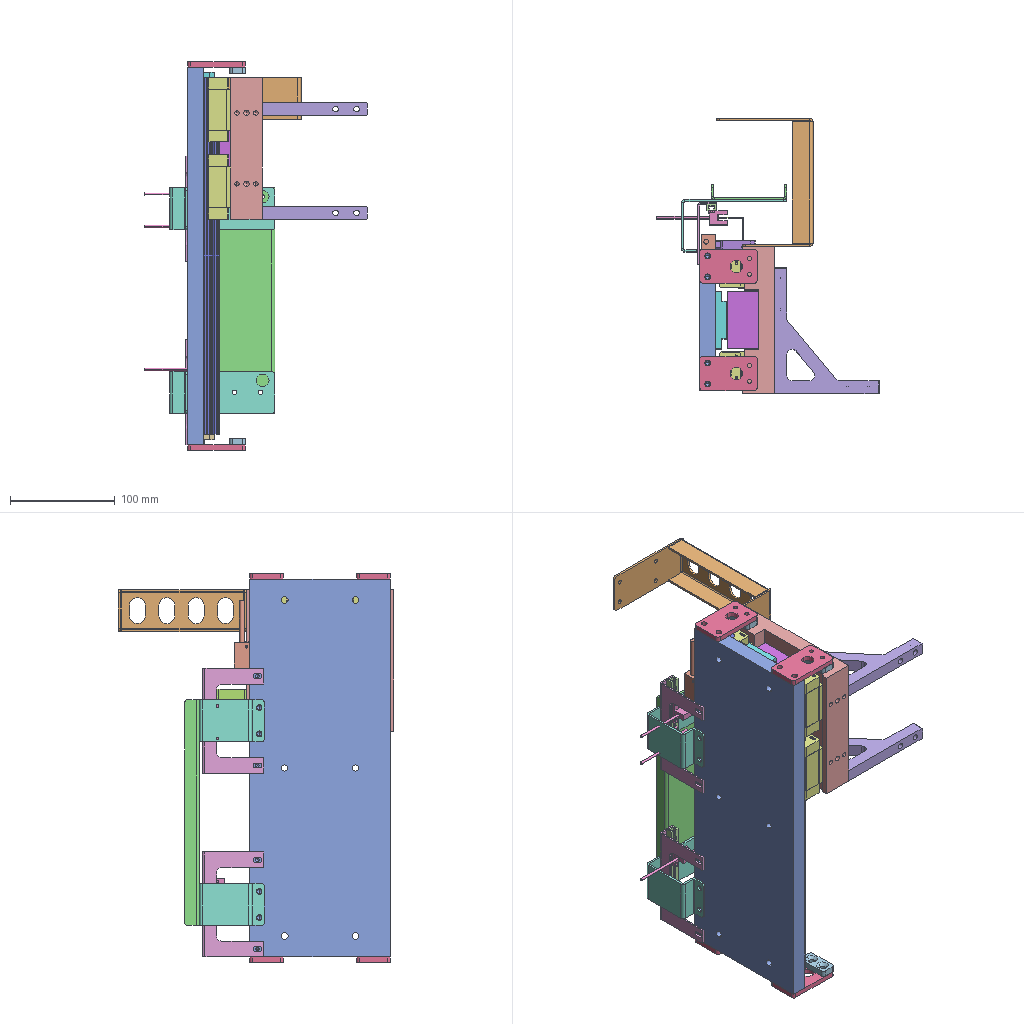Assembly | SolidWorks | 21 different items | 37 placed | box 212 x 262 x 370 mm
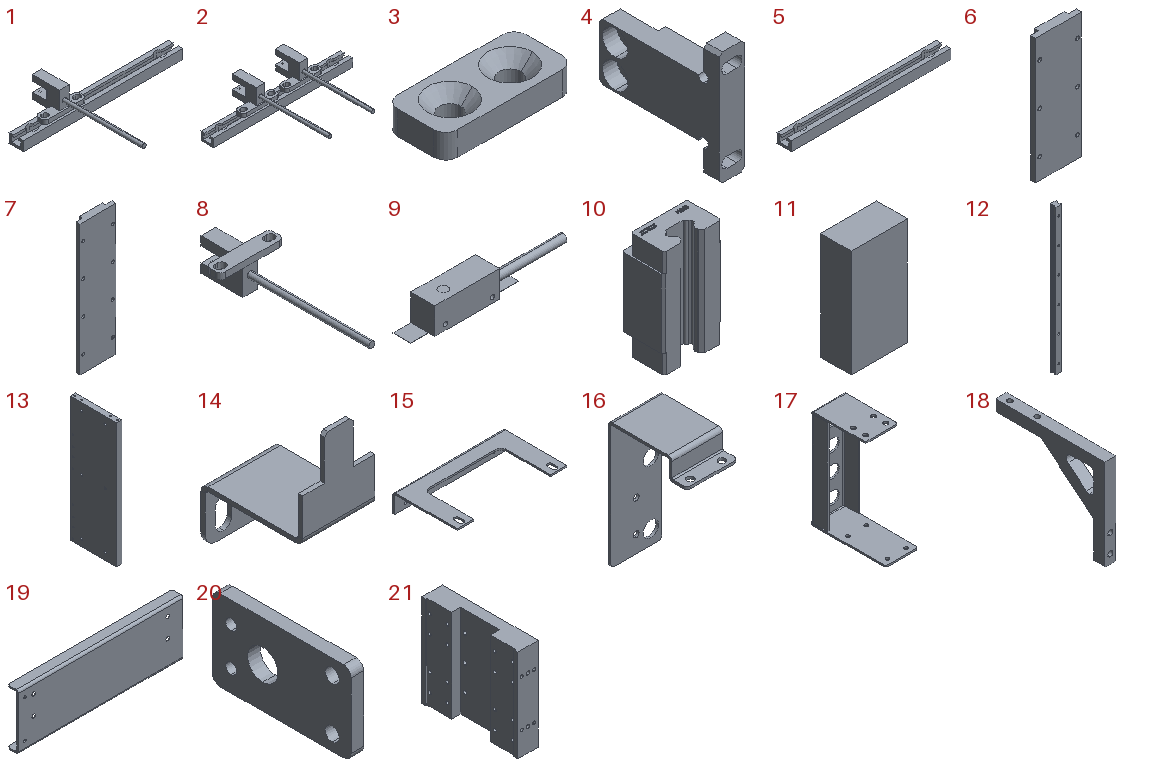Parts list (item | name | quantity | parent item | size | volume | features):
1 | (subassembly) | x1 | - | 100 x 67.2 x 19.7 mm | 4708 mm3 | -
2 | (subassembly) | x1 | - | 100 x 67.2 x 19.7 mm | 6293 mm3 | -
3 | - | x4 | - | 32 x 15 x 6 mm | 2360 mm3 | features Extrusion 1, Fillet 1, HoleWzd 1
4 | - | x1 | - | 8 x 38 x 36 mm | 4843 mm3 | features HoleWzd 2, ICE 2, Chamfer 1, Extrusion 1
5 | - | x2 | in 1, 2 | 100 x 9 x 6 mm | 3122 mm3 | features BaseBody 1
6 | - | x1 | - | 55 x 10.7 x 150 mm | 73163 mm3 | features BaseBody 1
7 | - | x1 | - | 55 x 10.7 x 200 mm | 97550 mm3 | features BaseBody 1
8 | - | x3 | in 1, 2 | 26 x 67.2 x 13.7 mm | 1586 mm3 | features BaseBody 1
9 | - | x1 | - | 86 x 13.4 x 14.9 mm | 7701 mm3 | features BaseBody 2
10 | - | x4 | - | 34 x 23.7 x 61.7 mm | 37046 mm3 | features BaseBody 1
11 | - | x1 | - | 55 x 30 x 120 mm | 172847 mm3 | features BaseBody 1
12 | - | x2 | - | 15 x 15 x 340 mm | 62525 mm3 | features Extrusion 1, HoleWzd 1, ICE 1, LPattern 1
13 | - | x1 | - | 15 x 134 x 360 mm | 714258 mm3 | features HoleWzd 7, LPattern 2, Extrusion 1, MirrorPattern 1
14 | - | x1 | - | 20 x 28.2 x 38 mm | 1272 mm3 | features Chamfer 1, Cut 1, Fillet 1, FlatPattern 1, HoleWzd 1, SMBaseFlange 1, SheetMetal 1
15 | - | x2 | - | 100 x 58.5 x 17.5 mm | 6237 mm3 | features HoleWzd 2, Cut 1, FlatPattern 1, SMBaseFlange 1, SheetMetal 1
16 | - | x2 | - | 40 x 62 x 100 mm | 13167 mm3 | features HoleWzd 3, Fillet 1, FlatPattern 1, SMBaseFlange 1, SheetMetal 1
17 | - | x1 | - | 40 x 92 x 122 mm | 27046 mm3 | features HoleWzd 2, EdgeFlange 1, Fillet 1, FlatPattern 1, ICE 1, LPattern 1, SMBaseFlange 1, SheetMetal 1
18 | - | x2 | - | 12 x 120 x 100 mm | 37463 mm3 | features HoleWzd 2, Chamfer 1, Extrusion 1, Fillet 1, ICE 1
19 | - | x1 | - | 215 x 14 x 72 mm | 40210 mm3 | features HoleWzd 2, Fillet 1, FlatPattern 1, SMBaseFlange 1, SheetMetal 1
20 | - | x4 | - | 5 x 55 x 32 mm | 7820 mm3 | features HoleWzd 2, Cut 1, Fillet 1, FlatPattern 1, SMBaseFlange 1, SheetMetal 1
21 | - | x1 | - | 30 x 140 x 135 mm | 401755 mm3 | features HoleWzd 8, ICE 2, Extrusion 1, LPattern 1
Mates (type | each side: item.copy, entity, surface, feature):
In the top assembly
Width | 10.1 face plane Input1 | 10.1 face plane Input1 | 12.1 face plane Boss-Extrude1 | 12.1 face plane Boss-Extrude1
Coincident | 12.1 face plane Boss-Extrude1 | 10.1 face plane Input1
Coincident | 10.1 face plane Input1 | 10.2 face plane Input1 | 2 times
DistanceDim | 10.2 face plane Input1 | 10.1 face plane Input1
Coincident | 10.1 face plane Input1 | 21.1 face plane Cut-Extrude2 | 2 times
Width | 10.1 face plane Input1 | 10.2 face plane Input1 | 21.1 face plane Boss-Extrude1 | 21.1 face plane Boss-Extrude1
Coincident | 10.2 face plane Input1 | 10.3 face plane Input1
Coincident | 21.1 face plane Cut-Extrude2 | 10.4 face plane Input1
LimitDistanceDim | 12.2 face plane Boss-Extrude1 | 21.1 face plane Boss-Extrude1
Coincident | 21.1 face plane Boss-Extrude1 | 14.1 face plane Base-Flange1 | 2 times
DistanceDim | 21.1 face plane Boss-Extrude1 | 14.1 face plane Base-Flange1
Coincident | 21.1 face plane Cut-Extrude1 | 11.1 face plane Input1
Width | 11.1 face plane Input1 | 11.1 face plane Input1 | 21.1 face plane Cut-Extrude1 | 21.1 face plane Cut-Extrude1
Width | 21.1 face plane Boss-Extrude1 | 21.1 face plane Boss-Extrude1 | 11.1 face plane Input1 | 11.1 face plane Input1
Width | 10.4 face plane Input1 | 10.4 face plane Input1 | 12.2 face plane Boss-Extrude1 | 12.2 face plane Boss-Extrude1
Coincident | 12.2 face plane Boss-Extrude1 | 10.4 face plane Input1
Width | 10.3 face plane Input1 | 10.3 face plane Input1 | 12.2 face plane Boss-Extrude1 | 12.2 face plane Boss-Extrude1
Coincident | 12.1 face plane Boss-Extrude1 | 12.2 face plane Boss-Extrude1
Coincident | 13.1 face plane Boss-Extrude1 | 12.2 face plane Boss-Extrude1
Width | 12.2 face plane Boss-Extrude1 | 12.1 face plane Boss-Extrude1 | 13.1 face plane Boss-Extrude1 | 13.1 face plane Boss-Extrude1
Coincident | 10.4 face plane Input1 | 10.3 face plane Input1
DistanceDim | 10.4 face plane Input1 | 10.3 face plane Input1
Coincident | 13.1 face plane Boss-Extrude1 | 9.1 face plane Input1
Coincident | 13.1 face plane Boss-Extrude1 | 12.1 face plane Boss-Extrude1
Width | 13.1 face plane Boss-Extrude1 | 13.1 face plane Boss-Extrude1 | 12.1 face plane Boss-Extrude1 | 12.1 face plane Boss-Extrude1
Coincident | 5.1 face plane Input1 | 5.2 face plane Input1 | 3 times
Coincident | 5.1 face plane Input1 | 15.1 face plane Base-Flange1 | 3 times
Width | 8.1 face plane Input1 | 8.1 face plane Input1 | 14.1 face plane Base-Flange1 | 14.1 face plane Base-Flange1
Coincident | 14.1 face plane Base-Flange1 | 8.1 face plane Input1
Coincident | 5.2 face plane Input1 | 15.2 face plane Base-Flange1 | 3 times
Width | 15.1 face plane Base-Flange1 | 15.1 face plane Base-Flange1 | 16.1 face plane Base-Flange1 | 16.1 face plane Base-Flange1
DistanceDim | 13.1 face plane Boss-Extrude1 | 15.1 face plane Base-Flange1
Coincident | 13.1 face plane Boss-Extrude1 | 15.2 face plane Base-Flange1
Coincident | 16.1 face plane Base-Flange1 | 16.2 face plane Base-Flange1
Coincident | 13.1 face plane Boss-Extrude1 | 16.1 face plane Base-Flange1 | 2 times
Coincident | 13.1 face plane Boss-Extrude1 | 16.2 face plane Base-Flange1
Coincident | 21.1 face plane Boss-Extrude1 | 17.1 face plane Base-Flange1 | 3 times
Coincident | 7.1 face plane Input1 | 6.1 face plane Input1 | 3 times
Coincident | 13.1 face plane Boss-Extrude1 | 7.1 face plane Input1
Width | 13.1 face plane Boss-Extrude1 | 13.1 face plane Boss-Extrude1 | 7.1 face plane Input1 | 7.1 face plane Input1
Coincident | 18.1 face plane Boss-Extrude1 | 18.2 face plane Boss-Extrude1
Coincident | 21.1 face plane Boss-Extrude1 | 18.1 face plane Boss-Extrude1 | 2 times
DistanceDim | 18.2 face plane Boss-Extrude1 | 21.1 face plane Boss-Extrude1
Width | 13.1 face plane Boss-Extrude1 | 13.1 face plane Boss-Extrude1 | 6.1 face plane Input1 | 7.1 face plane Input1
Coincident | 16.1 face plane Base-Flange1 | 19.1 face plane Base-Flange1 | 3 times
Coincident | 20.1 face plane Base-Flange1 | 3.1 face plane Boss-Extrude1
Concentric | 13.1 face cylinder M5 Tapped Hole1 | 20.1 face cylinder M5 Clearance Hole1 | 2 times
Coincident | 13.1 face plane Boss-Extrude1 | 20.1 face plane Base-Flange1
Coincident | 20.2 face plane Base-Flange1 | 3.2 face plane Boss-Extrude1
Concentric | 13.1 face cylinder M5 Tapped Hole1 | 20.2 face cylinder M5 Clearance Hole1 | 2 times
Coincident | 13.1 face plane Boss-Extrude1 | 20.2 face plane Base-Flange1
Coincident | 20.3 face plane Base-Flange1 | 3.3 face plane Boss-Extrude1
Concentric | 13.1 face cylinder Mirror1 | 20.3 face cylinder M5 Clearance Hole1 | 2 times
Coincident | 13.1 face plane Boss-Extrude1 | 20.3 face plane Base-Flange1
Coincident | 20.4 face plane Base-Flange1 | 3.4 face plane Boss-Extrude1
Concentric | 13.1 face cylinder Mirror1 | 20.4 face cylinder M5 Clearance Hole1 | 2 times
Coincident | 13.1 face plane Boss-Extrude1 | 20.4 face plane Base-Flange1
Width | 15.2 face plane Cut-Extrude1 | 15.2 face plane Cut-Extrude1 | 16.2 face plane Base-Flange1 | 16.2 face plane Base-Flange1
Concentric | 21.1 face cylinder M4 Tapped Hole1 | 4.1 face cylinder CBORE for M4 Hexagon socket head cap screws1 | 2 times
Coincident | 21.1 face plane Boss-Extrude1 | 4.1 face plane Cut-Extrude2
Concentric | 9.1 face cylinder Input2 | 4.1 face cylinder M3 clearance hole1
Coincident | 9.1 face plane Input2 | 4.1 face plane Boss-Extrude1
Concentric | 20.1 face cylinder M5 Tapped Hole1 | 3.1 face cylinder CSK for M5 Slotted raised CTSK head wood screws1 | 2 times
Concentric | 20.2 face cylinder M5 Tapped Hole1 | 3.2 face cylinder CSK for M5 Slotted raised CTSK head wood screws1 | 2 times
Concentric | 20.3 face cylinder M5 Tapped Hole1 | 3.3 face cylinder CSK for M5 Slotted raised CTSK head wood screws1 | 2 times
Concentric | 20.4 face cylinder M5 Tapped Hole1 | 3.4 face cylinder CSK for M5 Slotted raised CTSK head wood screws1 | 2 times
In subassembly 2
Coincident | 5.3 face plane Input1 | 8.2 face plane Input1
Width | 8.2 face plane Input1 | 8.2 face plane Input1 | 5.3 face plane Input1 | 5.3 face plane Input1
DistanceDim | 8.2 face plane Input1 | 5.3 face plane Input1
Coincident | 5.3 face plane Input1 | 8.3 face plane Input1
Width | 8.3 face plane Input1 | 8.3 face plane Input1 | 5.3 face plane Input1 | 5.3 face plane Input1
DistanceDim | 8.2 face plane Input1 | 8.3 face plane Input1
In subassembly 1
Coincident | 5.3 face plane Input1 | 8.2 face plane Input1
Width | 8.2 face plane Input1 | 8.2 face plane Input1 | 5.3 face plane Input1 | 5.3 face plane Input1
DistanceDim | 8.2 face plane Input1 | 5.3 face plane Input1